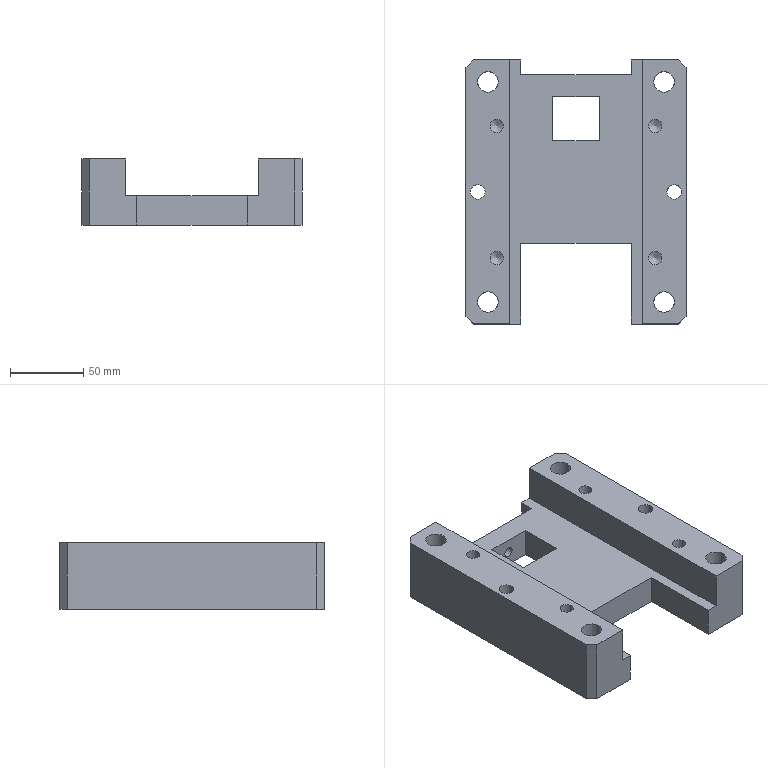Part | NX | features solid 2 | 1 solid | 43 faces | box 150 x 180 x 45 mm | volume 649811 mm3 | plane 27 | cylinder 12 | cone 4 | commonest cylinder face diameters 9 x4 14 x4 10 x2 7 x1 11 x1
STEP:
#1=CARTESIAN_POINT('',(45.,730.,-108.));
#2=VERTEX_POINT('',#1);
#3=CARTESIAN_POINT('',(70.,730.,-108.));
#4=VERTEX_POINT('',#3);
#5=CARTESIAN_POINT('',(45.,730.,-108.));
#6=DIRECTION('',(1.,0.,0.));
#7=VECTOR('',#6,1000.);
#8=LINE('',#5,#7);
#9=EDGE_CURVE('',#2,#4,#8,.T.);
#10=ORIENTED_EDGE('',*,*,#9,.T.);
#11=CARTESIAN_POINT('',(70.,730.,-153.));
#12=VERTEX_POINT('',#11);
#13=CARTESIAN_POINT('',(70.,730.,-153.));
#14=DIRECTION('',(0.,0.,-1.));
#15=VECTOR('',#14,1000.);
#16=LINE('',#13,#15);
#17=EDGE_CURVE('',#4,#12,#16,.T.);
#18=ORIENTED_EDGE('',*,*,#17,.T.);
#19=CARTESIAN_POINT('',(37.5,730.,-153.));
#20=VERTEX_POINT('',#19);
#21=CARTESIAN_POINT('',(75.,730.,-153.));
#22=DIRECTION('',(-1.,0.,0.));
#23=VECTOR('',#22,1000.);
#24=LINE('',#21,#23);
#25=EDGE_CURVE('',#12,#20,#24,.T.);
#26=ORIENTED_EDGE('',*,*,#25,.T.);
#27=CARTESIAN_POINT('',(37.5,730.,-133.));
#28=VERTEX_POINT('',#27);
#29=CARTESIAN_POINT('',(37.5,730.,-153.));
#30=DIRECTION('',(0.,0.,-1.));
#31=VECTOR('',#30,1000.);
#32=LINE('',#29,#31);
#33=EDGE_CURVE('',#28,#20,#32,.T.);
#34=ORIENTED_EDGE('',*,*,#33,.F.);
#35=CARTESIAN_POINT('',(45.,730.,-133.));
#36=VERTEX_POINT('',#35);
#37=CARTESIAN_POINT('',(-45.,730.,-133.));
#38=DIRECTION('',(1.,0.,0.));
#39=VECTOR('',#38,1000.);
#40=LINE('',#37,#39);
#41=EDGE_CURVE('',#28,#36,#40,.T.);
#42=ORIENTED_EDGE('',*,*,#41,.T.);
#43=CARTESIAN_POINT('',(45.,730.,-133.));
#44=DIRECTION('',(0.,0.,1.));
#45=VECTOR('',#44,1000.);
#46=LINE('',#43,#45);
#47=EDGE_CURVE('',#36,#2,#46,.T.);
#48=ORIENTED_EDGE('',*,*,#47,.T.);
#49=EDGE_LOOP('',(#10,#18,#26,#34,#42,#48));
#50=FACE_BOUND('',#49,.T.);
#51=CARTESIAN_POINT('',(45.,730.,-153.));
#52=DIRECTION('',(0.,-1.,0.));
#53=DIRECTION('',(0.,0.,-1.));
#54=AXIS2_PLACEMENT_3D('',#51,#52,#53);
#55=PLANE('',#54);
#56=ADVANCED_FACE('',(#50),#55,.F.);
#57=CARTESIAN_POINT('',(70.,550.,-153.));
#58=VERTEX_POINT('',#57);
#59=CARTESIAN_POINT('',(37.5,550.,-153.));
#60=VERTEX_POINT('',#59);
#61=CARTESIAN_POINT('',(75.,550.,-153.));
#62=DIRECTION('',(-1.,0.,0.));
#63=VECTOR('',#62,1000.);
#64=LINE('',#61,#63);
#65=EDGE_CURVE('',#58,#60,#64,.T.);
#66=ORIENTED_EDGE('',*,*,#65,.F.);
#67=CARTESIAN_POINT('',(70.,550.,-108.));
#68=VERTEX_POINT('',#67);
#69=CARTESIAN_POINT('',(70.,550.,-153.));
#70=DIRECTION('',(0.,0.,1.));
#71=VECTOR('',#70,1000.);
#72=LINE('',#69,#71);
#73=EDGE_CURVE('',#58,#68,#72,.T.);
#74=ORIENTED_EDGE('',*,*,#73,.T.);
#75=CARTESIAN_POINT('',(45.,550.,-108.));
#76=VERTEX_POINT('',#75);
#77=CARTESIAN_POINT('',(45.,550.,-108.));
#78=DIRECTION('',(1.,0.,0.));
#79=VECTOR('',#78,1000.);
#80=LINE('',#77,#79);
#81=EDGE_CURVE('',#76,#68,#80,.T.);
#82=ORIENTED_EDGE('',*,*,#81,.F.);
#83=CARTESIAN_POINT('',(45.,550.,-133.));
#84=VERTEX_POINT('',#83);
#85=CARTESIAN_POINT('',(45.,550.,-133.));
#86=DIRECTION('',(0.,0.,1.));
#87=VECTOR('',#86,1000.);
#88=LINE('',#85,#87);
#89=EDGE_CURVE('',#84,#76,#88,.T.);
#90=ORIENTED_EDGE('',*,*,#89,.F.);
#91=CARTESIAN_POINT('',(37.5,550.,-133.));
#92=VERTEX_POINT('',#91);
#93=CARTESIAN_POINT('',(-45.,550.,-133.));
#94=DIRECTION('',(1.,0.,0.));
#95=VECTOR('',#94,1000.);
#96=LINE('',#93,#95);
#97=EDGE_CURVE('',#92,#84,#96,.T.);
#98=ORIENTED_EDGE('',*,*,#97,.F.);
#99=CARTESIAN_POINT('',(37.5,550.,-153.));
#100=DIRECTION('',(0.,0.,-1.));
#101=VECTOR('',#100,1000.);
#102=LINE('',#99,#101);
#103=EDGE_CURVE('',#92,#60,#102,.T.);
#104=ORIENTED_EDGE('',*,*,#103,.T.);
#105=EDGE_LOOP('',(#66,#74,#82,#90,#98,#104));
#106=FACE_BOUND('',#105,.T.);
#107=CARTESIAN_POINT('',(45.,550.,-153.));
#108=DIRECTION('',(0.,-1.,0.));
#109=DIRECTION('',(0.,0.,-1.));
#110=AXIS2_PLACEMENT_3D('',#107,#108,#109);
#111=PLANE('',#110);
#112=ADVANCED_FACE('',(#106),#111,.T.);
#113=ORIENTED_EDGE('',*,*,#47,.F.);
#114=CARTESIAN_POINT('',(45.,550.,-133.));
#115=DIRECTION('',(0.,1.,0.));
#116=VECTOR('',#115,1000.);
#117=LINE('',#114,#116);
#118=EDGE_CURVE('',#84,#36,#117,.T.);
#119=ORIENTED_EDGE('',*,*,#118,.F.);
#120=ORIENTED_EDGE('',*,*,#89,.T.);
#121=CARTESIAN_POINT('',(45.,550.,-108.));
#122=DIRECTION('',(0.,1.,0.));
#123=VECTOR('',#122,1000.);
#124=LINE('',#121,#123);
#125=EDGE_CURVE('',#76,#2,#124,.T.);
#126=ORIENTED_EDGE('',*,*,#125,.T.);
#127=EDGE_LOOP('',(#113,#119,#120,#126));
#128=FACE_BOUND('',#127,.T.);
#129=CARTESIAN_POINT('',(45.,550.,-133.));
#130=DIRECTION('',(-1.,0.,0.));
#131=DIRECTION('',(0.,0.,-1.));
#132=AXIS2_PLACEMENT_3D('',#129,#130,#131);
#133=PLANE('',#132);
#134=ADVANCED_FACE('',(#128),#133,.T.);
#135=CARTESIAN_POINT('',(58.5,685.,-108.));
#136=VERTEX_POINT('',#135);
#137=CARTESIAN_POINT('',(54.,685.,-108.));
#138=DIRECTION('',(0.,0.,-1.));
#139=DIRECTION('',(1.,0.,0.));
#140=AXIS2_PLACEMENT_3D('',#137,#138,#139);
#141=CIRCLE('',#140,4.5);
#142=EDGE_CURVE('',#136,#136,#141,.T.);
#143=ORIENTED_EDGE('',*,*,#142,.T.);
#144=EDGE_LOOP('',(#143));
#145=FACE_BOUND('',#144,.T.);
#146=CARTESIAN_POINT('',(58.5,595.,-108.));
#147=VERTEX_POINT('',#146);
#148=CARTESIAN_POINT('',(54.,595.,-108.));
#149=DIRECTION('',(0.,0.,-1.));
#150=DIRECTION('',(1.,0.,0.));
#151=AXIS2_PLACEMENT_3D('',#148,#149,#150);
#152=CIRCLE('',#151,4.5);
#153=EDGE_CURVE('',#147,#147,#152,.T.);
#154=ORIENTED_EDGE('',*,*,#153,.T.);
#155=EDGE_LOOP('',(#154));
#156=FACE_BOUND('',#155,.T.);
#157=CARTESIAN_POINT('',(72.,640.,-108.));
#158=VERTEX_POINT('',#157);
#159=CARTESIAN_POINT('',(67.,640.,-108.));
#160=DIRECTION('',(0.,0.,-1.));
#161=DIRECTION('',(1.,0.,0.));
#162=AXIS2_PLACEMENT_3D('',#159,#160,#161);
#163=CIRCLE('',#162,5.);
#164=EDGE_CURVE('',#158,#158,#163,.T.);
#165=ORIENTED_EDGE('',*,*,#164,.T.);
#166=EDGE_LOOP('',(#165));
#167=FACE_BOUND('',#166,.T.);
#168=CARTESIAN_POINT('',(67.,565.,-108.));
#169=VERTEX_POINT('',#168);
#170=CARTESIAN_POINT('',(60.,565.,-108.));
#171=DIRECTION('',(0.,0.,-1.));
#172=DIRECTION('',(1.,0.,0.));
#173=AXIS2_PLACEMENT_3D('',#170,#171,#172);
#174=CIRCLE('',#173,7.);
#175=EDGE_CURVE('',#169,#169,#174,.T.);
#176=ORIENTED_EDGE('',*,*,#175,.T.);
#177=EDGE_LOOP('',(#176));
#178=FACE_BOUND('',#177,.T.);
#179=CARTESIAN_POINT('',(67.,715.,-108.));
#180=VERTEX_POINT('',#179);
#181=CARTESIAN_POINT('',(60.,715.,-108.));
#182=DIRECTION('',(0.,0.,-1.));
#183=DIRECTION('',(1.,0.,0.));
#184=AXIS2_PLACEMENT_3D('',#181,#182,#183);
#185=CIRCLE('',#184,7.);
#186=EDGE_CURVE('',#180,#180,#185,.T.);
#187=ORIENTED_EDGE('',*,*,#186,.T.);
#188=EDGE_LOOP('',(#187));
#189=FACE_BOUND('',#188,.T.);
#190=CARTESIAN_POINT('',(75.,555.,-108.));
#191=VERTEX_POINT('',#190);
#192=CARTESIAN_POINT('',(75.,725.,-108.));
#193=VERTEX_POINT('',#192);
#194=CARTESIAN_POINT('',(75.,550.,-108.));
#195=DIRECTION('',(0.,1.,0.));
#196=VECTOR('',#195,1000.);
#197=LINE('',#194,#196);
#198=EDGE_CURVE('',#191,#193,#197,.T.);
#199=ORIENTED_EDGE('',*,*,#198,.T.);
#200=CARTESIAN_POINT('',(147.5,652.5,-108.));
#201=DIRECTION('',(-0.7071,0.7071,0.));
#202=VECTOR('',#201,1000.);
#203=LINE('',#200,#202);
#204=EDGE_CURVE('',#193,#4,#203,.T.);
#205=ORIENTED_EDGE('',*,*,#204,.T.);
#206=ORIENTED_EDGE('',*,*,#9,.F.);
#207=ORIENTED_EDGE('',*,*,#125,.F.);
#208=ORIENTED_EDGE('',*,*,#81,.T.);
#209=CARTESIAN_POINT('',(57.5,537.5,-108.));
#210=DIRECTION('',(-0.7071,-0.7071,0.));
#211=VECTOR('',#210,1000.);
#212=LINE('',#209,#211);
#213=EDGE_CURVE('',#68,#191,#212,.F.);
#214=ORIENTED_EDGE('',*,*,#213,.T.);
#215=EDGE_LOOP('',(#199,#205,#206,#207,#208,#214));
#216=FACE_BOUND('',#215,.T.);
#217=CARTESIAN_POINT('',(45.,550.,-108.));
#218=DIRECTION('',(0.,0.,1.));
#219=DIRECTION('',(-1.,0.,0.));
#220=AXIS2_PLACEMENT_3D('',#217,#218,#219);
#221=PLANE('',#220);
#222=ADVANCED_FACE('',(#145,#156,#167,#178,#189,#216),#221,.T.);
#223=CARTESIAN_POINT('',(75.,555.,-153.));
#224=VERTEX_POINT('',#223);
#225=CARTESIAN_POINT('',(75.,725.,-153.));
#226=VERTEX_POINT('',#225);
#227=CARTESIAN_POINT('',(75.,550.,-153.));
#228=DIRECTION('',(0.,1.,0.));
#229=VECTOR('',#228,1000.);
#230=LINE('',#227,#229);
#231=EDGE_CURVE('',#224,#226,#230,.T.);
#232=ORIENTED_EDGE('',*,*,#231,.T.);
#233=CARTESIAN_POINT('',(75.,725.,-108.));
#234=DIRECTION('',(0.,0.,1.));
#235=VECTOR('',#234,1000.);
#236=LINE('',#233,#235);
#237=EDGE_CURVE('',#226,#193,#236,.T.);
#238=ORIENTED_EDGE('',*,*,#237,.T.);
#239=ORIENTED_EDGE('',*,*,#198,.F.);
#240=CARTESIAN_POINT('',(75.,555.,-108.));
#241=DIRECTION('',(0.,0.,-1.));
#242=VECTOR('',#241,1000.);
#243=LINE('',#240,#242);
#244=EDGE_CURVE('',#191,#224,#243,.T.);
#245=ORIENTED_EDGE('',*,*,#244,.T.);
#246=EDGE_LOOP('',(#232,#238,#239,#245));
#247=FACE_BOUND('',#246,.T.);
#248=CARTESIAN_POINT('',(75.,550.,-108.));
#249=DIRECTION('',(1.,0.,0.));
#250=DIRECTION('',(0.,0.,1.));
#251=AXIS2_PLACEMENT_3D('',#248,#249,#250);
#252=PLANE('',#251);
#253=ADVANCED_FACE('',(#247),#252,.T.);
#254=CARTESIAN_POINT('',(-67.,645.,-153.));
#255=VERTEX_POINT('',#254);
#256=CARTESIAN_POINT('',(-67.,640.,-153.));
#257=DIRECTION('',(0.,0.,-1.));
#258=DIRECTION('',(0.,1.,0.));
#259=AXIS2_PLACEMENT_3D('',#256,#257,#258);
#260=CIRCLE('',#259,5.);
#261=EDGE_CURVE('',#255,#255,#260,.T.);
#262=ORIENTED_EDGE('',*,*,#261,.F.);
#263=EDGE_LOOP('',(#262));
#264=FACE_BOUND('',#263,.T.);
#265=CARTESIAN_POINT('',(67.,645.,-153.));
#266=VERTEX_POINT('',#265);
#267=CARTESIAN_POINT('',(67.,640.,-153.));
#268=DIRECTION('',(0.,0.,-1.));
#269=DIRECTION('',(0.,1.,0.));
#270=AXIS2_PLACEMENT_3D('',#267,#268,#269);
#271=CIRCLE('',#270,5.);
#272=EDGE_CURVE('',#266,#266,#271,.T.);
#273=ORIENTED_EDGE('',*,*,#272,.F.);
#274=EDGE_LOOP('',(#273));
#275=FACE_BOUND('',#274,.T.);
#276=CARTESIAN_POINT('',(-60.,572.,-153.));
#277=VERTEX_POINT('',#276);
#278=CARTESIAN_POINT('',(-60.,565.,-153.));
#279=DIRECTION('',(0.,0.,-1.));
#280=DIRECTION('',(0.,1.,0.));
#281=AXIS2_PLACEMENT_3D('',#278,#279,#280);
#282=CIRCLE('',#281,7.);
#283=EDGE_CURVE('',#277,#277,#282,.T.);
#284=ORIENTED_EDGE('',*,*,#283,.F.);
#285=EDGE_LOOP('',(#284));
#286=FACE_BOUND('',#285,.T.);
#287=CARTESIAN_POINT('',(-60.,722.,-153.));
#288=VERTEX_POINT('',#287);
#289=CARTESIAN_POINT('',(-60.,715.,-153.));
#290=DIRECTION('',(0.,0.,-1.));
#291=DIRECTION('',(0.,1.,0.));
#292=AXIS2_PLACEMENT_3D('',#289,#290,#291);
#293=CIRCLE('',#292,7.);
#294=EDGE_CURVE('',#288,#288,#293,.T.);
#295=ORIENTED_EDGE('',*,*,#294,.F.);
#296=EDGE_LOOP('',(#295));
#297=FACE_BOUND('',#296,.T.);
#298=CARTESIAN_POINT('',(60.,572.,-153.));
#299=VERTEX_POINT('',#298);
#300=CARTESIAN_POINT('',(60.,565.,-153.));
#301=DIRECTION('',(0.,0.,-1.));
#302=DIRECTION('',(0.,1.,0.));
#303=AXIS2_PLACEMENT_3D('',#300,#301,#302);
#304=CIRCLE('',#303,7.);
#305=EDGE_CURVE('',#299,#299,#304,.T.);
#306=ORIENTED_EDGE('',*,*,#305,.F.);
#307=EDGE_LOOP('',(#306));
#308=FACE_BOUND('',#307,.T.);
#309=CARTESIAN_POINT('',(60.,722.,-153.));
#310=VERTEX_POINT('',#309);
#311=CARTESIAN_POINT('',(60.,715.,-153.));
#312=DIRECTION('',(0.,0.,-1.));
#313=DIRECTION('',(0.,1.,0.));
#314=AXIS2_PLACEMENT_3D('',#311,#312,#313);
#315=CIRCLE('',#314,7.);
#316=EDGE_CURVE('',#310,#310,#315,.T.);
#317=ORIENTED_EDGE('',*,*,#316,.F.);
#318=EDGE_LOOP('',(#317));
#319=FACE_BOUND('',#318,.T.);
#320=CARTESIAN_POINT('',(16.,675.,-153.));
#321=VERTEX_POINT('',#320);
#322=CARTESIAN_POINT('',(16.,705.,-153.));
#323=VERTEX_POINT('',#322);
#324=CARTESIAN_POINT('',(16.,675.,-153.));
#325=DIRECTION('',(0.,1.,0.));
#326=VECTOR('',#325,1000.);
#327=LINE('',#324,#326);
#328=EDGE_CURVE('',#321,#323,#327,.T.);
#329=ORIENTED_EDGE('',*,*,#328,.T.);
#330=CARTESIAN_POINT('',(-16.,705.,-153.));
#331=VERTEX_POINT('',#330);
#332=CARTESIAN_POINT('',(16.,705.,-153.));
#333=DIRECTION('',(-1.,0.,0.));
#334=VECTOR('',#333,1000.);
#335=LINE('',#332,#334);
#336=EDGE_CURVE('',#323,#331,#335,.T.);
#337=ORIENTED_EDGE('',*,*,#336,.T.);
#338=CARTESIAN_POINT('',(-16.,675.,-153.));
#339=VERTEX_POINT('',#338);
#340=CARTESIAN_POINT('',(-16.,675.,-153.));
#341=DIRECTION('',(0.,1.,0.));
#342=VECTOR('',#341,1000.);
#343=LINE('',#340,#342);
#344=EDGE_CURVE('',#339,#331,#343,.T.);
#345=ORIENTED_EDGE('',*,*,#344,.F.);
#346=CARTESIAN_POINT('',(16.,675.,-153.));
#347=DIRECTION('',(-1.,0.,0.));
#348=VECTOR('',#347,1000.);
#349=LINE('',#346,#348);
#350=EDGE_CURVE('',#321,#339,#349,.T.);
#351=ORIENTED_EDGE('',*,*,#350,.F.);
#352=EDGE_LOOP('',(#329,#337,#345,#351));
#353=FACE_BOUND('',#352,.T.);
#354=ORIENTED_EDGE('',*,*,#25,.F.);
#355=CARTESIAN_POINT('',(162.5,637.5,-153.));
#356=DIRECTION('',(0.7071,-0.7071,0.));
#357=VECTOR('',#356,1000.);
#358=LINE('',#355,#357);
#359=EDGE_CURVE('',#12,#226,#358,.T.);
#360=ORIENTED_EDGE('',*,*,#359,.T.);
#361=ORIENTED_EDGE('',*,*,#231,.F.);
#362=CARTESIAN_POINT('',(72.5,552.5,-153.));
#363=DIRECTION('',(0.7071,0.7071,0.));
#364=VECTOR('',#363,1000.);
#365=LINE('',#362,#364);
#366=EDGE_CURVE('',#224,#58,#365,.F.);
#367=ORIENTED_EDGE('',*,*,#366,.T.);
#368=ORIENTED_EDGE('',*,*,#65,.T.);
#369=CARTESIAN_POINT('',(37.5,605.,-153.));
#370=VERTEX_POINT('',#369);
#371=CARTESIAN_POINT('',(37.5,550.,-153.));
#372=DIRECTION('',(0.,1.,0.));
#373=VECTOR('',#372,1000.);
#374=LINE('',#371,#373);
#375=EDGE_CURVE('',#60,#370,#374,.T.);
#376=ORIENTED_EDGE('',*,*,#375,.T.);
#377=CARTESIAN_POINT('',(-37.5,605.,-153.));
#378=VERTEX_POINT('',#377);
#379=CARTESIAN_POINT('',(37.5,605.,-153.));
#380=DIRECTION('',(-1.,0.,0.));
#381=VECTOR('',#380,1000.);
#382=LINE('',#379,#381);
#383=EDGE_CURVE('',#370,#378,#382,.T.);
#384=ORIENTED_EDGE('',*,*,#383,.T.);
#385=CARTESIAN_POINT('',(-37.5,550.,-153.));
#386=VERTEX_POINT('',#385);
#387=CARTESIAN_POINT('',(-37.5,550.,-153.));
#388=DIRECTION('',(0.,1.,0.));
#389=VECTOR('',#388,1000.);
#390=LINE('',#387,#389);
#391=EDGE_CURVE('',#386,#378,#390,.T.);
#392=ORIENTED_EDGE('',*,*,#391,.F.);
#393=CARTESIAN_POINT('',(-70.,550.,-153.));
#394=VERTEX_POINT('',#393);
#395=CARTESIAN_POINT('',(75.,550.,-153.));
#396=DIRECTION('',(-1.,0.,0.));
#397=VECTOR('',#396,1000.);
#398=LINE('',#395,#397);
#399=EDGE_CURVE('',#386,#394,#398,.T.);
#400=ORIENTED_EDGE('',*,*,#399,.T.);
#401=CARTESIAN_POINT('',(-75.,555.,-153.));
#402=VERTEX_POINT('',#401);
#403=CARTESIAN_POINT('',(2.5,477.5,-153.));
#404=DIRECTION('',(0.7071,-0.7071,0.));
#405=VECTOR('',#404,1000.);
#406=LINE('',#403,#405);
#407=EDGE_CURVE('',#394,#402,#406,.F.);
#408=ORIENTED_EDGE('',*,*,#407,.T.);
#409=CARTESIAN_POINT('',(-75.,725.,-153.));
#410=VERTEX_POINT('',#409);
#411=CARTESIAN_POINT('',(-75.,550.,-153.));
#412=DIRECTION('',(0.,1.,0.));
#413=VECTOR('',#412,1000.);
#414=LINE('',#411,#413);
#415=EDGE_CURVE('',#402,#410,#414,.T.);
#416=ORIENTED_EDGE('',*,*,#415,.T.);
#417=CARTESIAN_POINT('',(-70.,730.,-153.));
#418=VERTEX_POINT('',#417);
#419=CARTESIAN_POINT('',(-87.5,712.5,-153.));
#420=DIRECTION('',(0.7071,0.7071,0.));
#421=VECTOR('',#420,1000.);
#422=LINE('',#419,#421);
#423=EDGE_CURVE('',#410,#418,#422,.T.);
#424=ORIENTED_EDGE('',*,*,#423,.T.);
#425=CARTESIAN_POINT('',(-37.5,730.,-153.));
#426=VERTEX_POINT('',#425);
#427=CARTESIAN_POINT('',(75.,730.,-153.));
#428=DIRECTION('',(-1.,0.,0.));
#429=VECTOR('',#428,1000.);
#430=LINE('',#427,#429);
#431=EDGE_CURVE('',#426,#418,#430,.T.);
#432=ORIENTED_EDGE('',*,*,#431,.F.);
#433=CARTESIAN_POINT('',(-37.5,720.,-153.));
#434=VERTEX_POINT('',#433);
#435=CARTESIAN_POINT('',(-37.5,720.,-153.));
#436=DIRECTION('',(0.,1.,0.));
#437=VECTOR('',#436,1000.);
#438=LINE('',#435,#437);
#439=EDGE_CURVE('',#434,#426,#438,.T.);
#440=ORIENTED_EDGE('',*,*,#439,.F.);
#441=CARTESIAN_POINT('',(37.5,720.,-153.));
#442=VERTEX_POINT('',#441);
#443=CARTESIAN_POINT('',(37.5,720.,-153.));
#444=DIRECTION('',(-1.,0.,0.));
#445=VECTOR('',#444,1000.);
#446=LINE('',#443,#445);
#447=EDGE_CURVE('',#442,#434,#446,.T.);
#448=ORIENTED_EDGE('',*,*,#447,.F.);
#449=CARTESIAN_POINT('',(37.5,720.,-153.));
#450=DIRECTION('',(0.,1.,0.));
#451=VECTOR('',#450,1000.);
#452=LINE('',#449,#451);
#453=EDGE_CURVE('',#442,#20,#452,.T.);
#454=ORIENTED_EDGE('',*,*,#453,.T.);
#455=EDGE_LOOP('',(#354,#360,#361,#367,#368,#376,#384,#392,#400,#408,#416,#424,#432,#440,#448,#454));
#456=FACE_BOUND('',#455,.T.);
#457=CARTESIAN_POINT('',(75.,550.,-153.));
#458=DIRECTION('',(0.,0.,-1.));
#459=DIRECTION('',(0.,1.,0.));
#460=AXIS2_PLACEMENT_3D('',#457,#458,#459);
#461=PLANE('',#460);
#462=ADVANCED_FACE('',(#264,#275,#286,#297,#308,#319,#353,#456),#461,.T.);
#463=CARTESIAN_POINT('',(-75.,555.,-108.));
#464=VERTEX_POINT('',#463);
#465=CARTESIAN_POINT('',(-75.,725.,-108.));
#466=VERTEX_POINT('',#465);
#467=CARTESIAN_POINT('',(-75.,550.,-108.));
#468=DIRECTION('',(0.,1.,0.));
#469=VECTOR('',#468,1000.);
#470=LINE('',#467,#469);
#471=EDGE_CURVE('',#464,#466,#470,.T.);
#472=ORIENTED_EDGE('',*,*,#471,.T.);
#473=CARTESIAN_POINT('',(-75.,725.,-153.));
#474=DIRECTION('',(0.,0.,-1.));
#475=VECTOR('',#474,1000.);
#476=LINE('',#473,#475);
#477=EDGE_CURVE('',#466,#410,#476,.T.);
#478=ORIENTED_EDGE('',*,*,#477,.T.);
#479=ORIENTED_EDGE('',*,*,#415,.F.);
#480=CARTESIAN_POINT('',(-75.,555.,-153.));
#481=DIRECTION('',(0.,0.,1.));
#482=VECTOR('',#481,1000.);
#483=LINE('',#480,#482);
#484=EDGE_CURVE('',#402,#464,#483,.T.);
#485=ORIENTED_EDGE('',*,*,#484,.T.);
#486=EDGE_LOOP('',(#472,#478,#479,#485));
#487=FACE_BOUND('',#486,.T.);
#488=CARTESIAN_POINT('',(-75.,550.,-153.));
#489=DIRECTION('',(-1.,0.,0.));
#490=DIRECTION('',(0.,0.,-1.));
#491=AXIS2_PLACEMENT_3D('',#488,#489,#490);
#492=PLANE('',#491);
#493=ADVANCED_FACE('',(#487),#492,.T.);
#494=CARTESIAN_POINT('',(-49.5,685.,-108.));
#495=VERTEX_POINT('',#494);
#496=CARTESIAN_POINT('',(-54.,685.,-108.));
#497=DIRECTION('',(0.,0.,-1.));
#498=DIRECTION('',(1.,0.,0.));
#499=AXIS2_PLACEMENT_3D('',#496,#497,#498);
#500=CIRCLE('',#499,4.5);
#501=EDGE_CURVE('',#495,#495,#500,.T.);
#502=ORIENTED_EDGE('',*,*,#501,.T.);
#503=EDGE_LOOP('',(#502));
#504=FACE_BOUND('',#503,.T.);
#505=CARTESIAN_POINT('',(-49.5,595.,-108.));
#506=VERTEX_POINT('',#505);
#507=CARTESIAN_POINT('',(-54.,595.,-108.));
#508=DIRECTION('',(0.,0.,-1.));
#509=DIRECTION('',(1.,0.,0.));
#510=AXIS2_PLACEMENT_3D('',#507,#508,#509);
#511=CIRCLE('',#510,4.5);
#512=EDGE_CURVE('',#506,#506,#511,.T.);
#513=ORIENTED_EDGE('',*,*,#512,.T.);
#514=EDGE_LOOP('',(#513));
#515=FACE_BOUND('',#514,.T.);
#516=CARTESIAN_POINT('',(-62.,640.,-108.));
#517=VERTEX_POINT('',#516);
#518=CARTESIAN_POINT('',(-67.,640.,-108.));
#519=DIRECTION('',(0.,0.,-1.));
#520=DIRECTION('',(1.,0.,0.));
#521=AXIS2_PLACEMENT_3D('',#518,#519,#520);
#522=CIRCLE('',#521,5.);
#523=EDGE_CURVE('',#517,#517,#522,.T.);
#524=ORIENTED_EDGE('',*,*,#523,.T.);
#525=EDGE_LOOP('',(#524));
#526=FACE_BOUND('',#525,.T.);
#527=CARTESIAN_POINT('',(-53.,565.,-108.));
#528=VERTEX_POINT('',#527);
#529=CARTESIAN_POINT('',(-60.,565.,-108.));
#530=DIRECTION('',(0.,0.,-1.));
#531=DIRECTION('',(1.,0.,0.));
#532=AXIS2_PLACEMENT_3D('',#529,#530,#531);
#533=CIRCLE('',#532,7.);
#534=EDGE_CURVE('',#528,#528,#533,.T.);
#535=ORIENTED_EDGE('',*,*,#534,.T.);
#536=EDGE_LOOP('',(#535));
#537=FACE_BOUND('',#536,.T.);
#538=CARTESIAN_POINT('',(-53.,715.,-108.));
#539=VERTEX_POINT('',#538);
#540=CARTESIAN_POINT('',(-60.,715.,-108.));
#541=DIRECTION('',(0.,0.,-1.));
#542=DIRECTION('',(1.,0.,0.));
#543=AXIS2_PLACEMENT_3D('',#540,#541,#542);
#544=CIRCLE('',#543,7.);
#545=EDGE_CURVE('',#539,#539,#544,.T.);
#546=ORIENTED_EDGE('',*,*,#545,.T.);
#547=EDGE_LOOP('',(#546));
#548=FACE_BOUND('',#547,.T.);
#549=CARTESIAN_POINT('',(-70.,730.,-108.));
#550=VERTEX_POINT('',#549);
#551=CARTESIAN_POINT('',(-45.,730.,-108.));
#552=VERTEX_POINT('',#551);
#553=CARTESIAN_POINT('',(-75.,730.,-108.));
#554=DIRECTION('',(1.,0.,0.));
#555=VECTOR('',#554,1000.);
#556=LINE('',#553,#555);
#557=EDGE_CURVE('',#550,#552,#556,.T.);
#558=ORIENTED_EDGE('',*,*,#557,.F.);
#559=CARTESIAN_POINT('',(-162.5,637.5,-108.));
#560=DIRECTION('',(-0.7071,-0.7071,0.));
#561=VECTOR('',#560,1000.);
#562=LINE('',#559,#561);
#563=EDGE_CURVE('',#550,#466,#562,.T.);
#564=ORIENTED_EDGE('',*,*,#563,.T.);
#565=ORIENTED_EDGE('',*,*,#471,.F.);
#566=CARTESIAN_POINT('',(-70.,550.,-108.));
#567=VERTEX_POINT('',#566);
#568=CARTESIAN_POINT('',(-72.5,552.5,-108.));
#569=DIRECTION('',(-0.7071,0.7071,0.));
#570=VECTOR('',#569,1000.);
#571=LINE('',#568,#570);
#572=EDGE_CURVE('',#464,#567,#571,.F.);
#573=ORIENTED_EDGE('',*,*,#572,.T.);
#574=CARTESIAN_POINT('',(-45.,550.,-108.));
#575=VERTEX_POINT('',#574);
#576=CARTESIAN_POINT('',(-75.,550.,-108.));
#577=DIRECTION('',(1.,0.,0.));
#578=VECTOR('',#577,1000.);
#579=LINE('',#576,#578);
#580=EDGE_CURVE('',#567,#575,#579,.T.);
#581=ORIENTED_EDGE('',*,*,#580,.T.);
#582=CARTESIAN_POINT('',(-45.,550.,-108.));
#583=DIRECTION('',(0.,1.,0.));
#584=VECTOR('',#583,1000.);
#585=LINE('',#582,#584);
#586=EDGE_CURVE('',#575,#552,#585,.T.);
#587=ORIENTED_EDGE('',*,*,#586,.T.);
#588=EDGE_LOOP('',(#558,#564,#565,#573,#581,#587));
#589=FACE_BOUND('',#588,.T.);
#590=CARTESIAN_POINT('',(-75.,550.,-108.));
#591=DIRECTION('',(0.,0.,1.));
#592=DIRECTION('',(0.,-1.,0.));
#593=AXIS2_PLACEMENT_3D('',#590,#591,#592);
#594=PLANE('',#593);
#595=ADVANCED_FACE('',(#504,#515,#526,#537,#548,#589),#594,.T.);
#596=CARTESIAN_POINT('',(-45.,730.,-133.));
#597=VERTEX_POINT('',#596);
#598=CARTESIAN_POINT('',(-45.,730.,-108.));
#599=DIRECTION('',(0.,0.,-1.));
#600=VECTOR('',#599,1000.);
#601=LINE('',#598,#600);
#602=EDGE_CURVE('',#552,#597,#601,.T.);
#603=ORIENTED_EDGE('',*,*,#602,.F.);
#604=ORIENTED_EDGE('',*,*,#586,.F.);
#605=CARTESIAN_POINT('',(-45.,550.,-133.));
#606=VERTEX_POINT('',#605);
#607=CARTESIAN_POINT('',(-45.,550.,-108.));
#608=DIRECTION('',(0.,0.,-1.));
#609=VECTOR('',#608,1000.);
#610=LINE('',#607,#609);
#611=EDGE_CURVE('',#575,#606,#610,.T.);
#612=ORIENTED_EDGE('',*,*,#611,.T.);
#613=CARTESIAN_POINT('',(-45.,550.,-133.));
#614=DIRECTION('',(0.,1.,0.));
#615=VECTOR('',#614,1000.);
#616=LINE('',#613,#615);
#617=EDGE_CURVE('',#606,#597,#616,.T.);
#618=ORIENTED_EDGE('',*,*,#617,.T.);
#619=EDGE_LOOP('',(#603,#604,#612,#618));
#620=FACE_BOUND('',#619,.T.);
#621=CARTESIAN_POINT('',(-45.,550.,-108.));
#622=DIRECTION('',(1.,0.,0.));
#623=DIRECTION('',(0.,0.,1.));
#624=AXIS2_PLACEMENT_3D('',#621,#622,#623);
#625=PLANE('',#624);
#626=ADVANCED_FACE('',(#620),#625,.T.);
#627=CARTESIAN_POINT('',(16.,675.,-133.));
#628=VERTEX_POINT('',#627);
#629=CARTESIAN_POINT('',(16.,705.,-133.));
#630=VERTEX_POINT('',#629);
#631=CARTESIAN_POINT('',(16.,675.,-133.));
#632=DIRECTION('',(0.,1.,0.));
#633=VECTOR('',#632,1000.);
#634=LINE('',#631,#633);
#635=EDGE_CURVE('',#628,#630,#634,.T.);
#636=ORIENTED_EDGE('',*,*,#635,.F.);
#637=CARTESIAN_POINT('',(-16.,675.,-133.));
#638=VERTEX_POINT('',#637);
#639=CARTESIAN_POINT('',(16.,675.,-133.));
#640=DIRECTION('',(-1.,0.,0.));
#641=VECTOR('',#640,1000.);
#642=LINE('',#639,#641);
#643=EDGE_CURVE('',#628,#638,#642,.T.);
#644=ORIENTED_EDGE('',*,*,#643,.T.);
#645=CARTESIAN_POINT('',(-16.,705.,-133.));
#646=VERTEX_POINT('',#645);
#647=CARTESIAN_POINT('',(-16.,675.,-133.));
#648=DIRECTION('',(0.,1.,0.));
#649=VECTOR('',#648,1000.);
#650=LINE('',#647,#649);
#651=EDGE_CURVE('',#638,#646,#650,.T.);
#652=ORIENTED_EDGE('',*,*,#651,.T.);
#653=CARTESIAN_POINT('',(16.,705.,-133.));
#654=DIRECTION('',(-1.,0.,0.));
#655=VECTOR('',#654,1000.);
#656=LINE('',#653,#655);
#657=EDGE_CURVE('',#630,#646,#656,.T.);
#658=ORIENTED_EDGE('',*,*,#657,.F.);
#659=EDGE_LOOP('',(#636,#644,#652,#658));
#660=FACE_BOUND('',#659,.T.);
#661=CARTESIAN_POINT('',(37.5,720.,-133.));
#662=VERTEX_POINT('',#661);
#663=CARTESIAN_POINT('',(37.5,720.,-133.));
#664=DIRECTION('',(0.,1.,0.));
#665=VECTOR('',#664,1000.);
#666=LINE('',#663,#665);
#667=EDGE_CURVE('',#662,#28,#666,.T.);
#668=ORIENTED_EDGE('',*,*,#667,.F.);
#669=CARTESIAN_POINT('',(-37.5,720.,-133.));
#670=VERTEX_POINT('',#669);
#671=CARTESIAN_POINT('',(37.5,720.,-133.));
#672=DIRECTION('',(-1.,0.,0.));
#673=VECTOR('',#672,1000.);
#674=LINE('',#671,#673);
#675=EDGE_CURVE('',#662,#670,#674,.T.);
#676=ORIENTED_EDGE('',*,*,#675,.T.);
#677=CARTESIAN_POINT('',(-37.5,730.,-133.));
#678=VERTEX_POINT('',#677);
#679=CARTESIAN_POINT('',(-37.5,720.,-133.));
#680=DIRECTION('',(0.,1.,0.));
#681=VECTOR('',#680,1000.);
#682=LINE('',#679,#681);
#683=EDGE_CURVE('',#670,#678,#682,.T.);
#684=ORIENTED_EDGE('',*,*,#683,.T.);
#685=CARTESIAN_POINT('',(-45.,730.,-133.));
#686=DIRECTION('',(1.,0.,0.));
#687=VECTOR('',#686,1000.);
#688=LINE('',#685,#687);
#689=EDGE_CURVE('',#597,#678,#688,.T.);
#690=ORIENTED_EDGE('',*,*,#689,.F.);
#691=ORIENTED_EDGE('',*,*,#617,.F.);
#692=CARTESIAN_POINT('',(-37.5,550.,-133.));
#693=VERTEX_POINT('',#692);
#694=CARTESIAN_POINT('',(-45.,550.,-133.));
#695=DIRECTION('',(1.,0.,0.));
#696=VECTOR('',#695,1000.);
#697=LINE('',#694,#696);
#698=EDGE_CURVE('',#606,#693,#697,.T.);
#699=ORIENTED_EDGE('',*,*,#698,.T.);
#700=CARTESIAN_POINT('',(-37.5,605.,-133.));
#701=VERTEX_POINT('',#700);
#702=CARTESIAN_POINT('',(-37.5,550.,-133.));
#703=DIRECTION('',(0.,1.,0.));
#704=VECTOR('',#703,1000.);
#705=LINE('',#702,#704);
#706=EDGE_CURVE('',#693,#701,#705,.T.);
#707=ORIENTED_EDGE('',*,*,#706,.T.);
#708=CARTESIAN_POINT('',(37.5,605.,-133.));
#709=VERTEX_POINT('',#708);
#710=CARTESIAN_POINT('',(37.5,605.,-133.));
#711=DIRECTION('',(-1.,0.,0.));
#712=VECTOR('',#711,1000.);
#713=LINE('',#710,#712);
#714=EDGE_CURVE('',#709,#701,#713,.T.);
#715=ORIENTED_EDGE('',*,*,#714,.F.);
#716=CARTESIAN_POINT('',(37.5,550.,-133.));
#717=DIRECTION('',(0.,1.,0.));
#718=VECTOR('',#717,1000.);
#719=LINE('',#716,#718);
#720=EDGE_CURVE('',#92,#709,#719,.T.);
#721=ORIENTED_EDGE('',*,*,#720,.F.);
#722=ORIENTED_EDGE('',*,*,#97,.T.);
#723=ORIENTED_EDGE('',*,*,#118,.T.);
#724=ORIENTED_EDGE('',*,*,#41,.F.);
#725=EDGE_LOOP('',(#668,#676,#684,#690,#691,#699,#707,#715,#721,#722,#723,#724));
#726=FACE_BOUND('',#725,.T.);
#727=CARTESIAN_POINT('',(-45.,550.,-133.));
#728=DIRECTION('',(0.,0.,1.));
#729=DIRECTION('',(-1.,0.,0.));
#730=AXIS2_PLACEMENT_3D('',#727,#728,#729);
#731=PLANE('',#730);
#732=ADVANCED_FACE('',(#660,#726),#731,.T.);
#733=ORIENTED_EDGE('',*,*,#580,.F.);
#734=CARTESIAN_POINT('',(-70.,550.,-153.));
#735=DIRECTION('',(0.,0.,-1.));
#736=VECTOR('',#735,1000.);
#737=LINE('',#734,#736);
#738=EDGE_CURVE('',#567,#394,#737,.T.);
#739=ORIENTED_EDGE('',*,*,#738,.T.);
#740=ORIENTED_EDGE('',*,*,#399,.F.);
#741=CARTESIAN_POINT('',(-37.5,550.,-153.));
#742=DIRECTION('',(0.,0.,-1.));
#743=VECTOR('',#742,1000.);
#744=LINE('',#741,#743);
#745=EDGE_CURVE('',#693,#386,#744,.T.);
#746=ORIENTED_EDGE('',*,*,#745,.F.);
#747=ORIENTED_EDGE('',*,*,#698,.F.);
#748=ORIENTED_EDGE('',*,*,#611,.F.);
#749=EDGE_LOOP('',(#733,#739,#740,#746,#747,#748));
#750=FACE_BOUND('',#749,.T.);
#751=CARTESIAN_POINT('',(45.,550.,-153.));
#752=DIRECTION('',(0.,-1.,0.));
#753=DIRECTION('',(0.,0.,-1.));
#754=AXIS2_PLACEMENT_3D('',#751,#752,#753);
#755=PLANE('',#754);
#756=ADVANCED_FACE('',(#750),#755,.T.);
#757=ORIENTED_EDGE('',*,*,#431,.T.);
#758=CARTESIAN_POINT('',(-70.,730.,-108.));
#759=DIRECTION('',(0.,0.,1.));
#760=VECTOR('',#759,1000.);
#761=LINE('',#758,#760);
#762=EDGE_CURVE('',#418,#550,#761,.T.);
#763=ORIENTED_EDGE('',*,*,#762,.T.);
#764=ORIENTED_EDGE('',*,*,#557,.T.);
#765=ORIENTED_EDGE('',*,*,#602,.T.);
#766=ORIENTED_EDGE('',*,*,#689,.T.);
#767=CARTESIAN_POINT('',(-37.5,730.,-153.));
#768=DIRECTION('',(0.,0.,-1.));
#769=VECTOR('',#768,1000.);
#770=LINE('',#767,#769);
#771=EDGE_CURVE('',#678,#426,#770,.T.);
#772=ORIENTED_EDGE('',*,*,#771,.T.);
#773=EDGE_LOOP('',(#757,#763,#764,#765,#766,#772));
#774=FACE_BOUND('',#773,.T.);
#775=CARTESIAN_POINT('',(45.,730.,-153.));
#776=DIRECTION('',(0.,-1.,0.));
#777=DIRECTION('',(0.,0.,-1.));
#778=AXIS2_PLACEMENT_3D('',#775,#776,#777);
#779=PLANE('',#778);
#780=ADVANCED_FACE('',(#774),#779,.F.);
#781=ORIENTED_EDGE('',*,*,#720,.T.);
#782=CARTESIAN_POINT('',(37.5,605.,-153.));
#783=DIRECTION('',(0.,0.,-1.));
#784=VECTOR('',#783,1000.);
#785=LINE('',#782,#784);
#786=EDGE_CURVE('',#709,#370,#785,.T.);
#787=ORIENTED_EDGE('',*,*,#786,.T.);
#788=ORIENTED_EDGE('',*,*,#375,.F.);
#789=ORIENTED_EDGE('',*,*,#103,.F.);
#790=EDGE_LOOP('',(#781,#787,#788,#789));
#791=FACE_BOUND('',#790,.T.);
#792=CARTESIAN_POINT('',(37.5,550.,-133.));
#793=DIRECTION('',(1.,0.,0.));
#794=DIRECTION('',(0.,0.,1.));
#795=AXIS2_PLACEMENT_3D('',#792,#793,#794);
#796=PLANE('',#795);
#797=ADVANCED_FACE('',(#791),#796,.F.);
#798=ORIENTED_EDGE('',*,*,#714,.T.);
#799=CARTESIAN_POINT('',(-37.5,605.,-153.));
#800=DIRECTION('',(0.,0.,-1.));
#801=VECTOR('',#800,1000.);
#802=LINE('',#799,#801);
#803=EDGE_CURVE('',#701,#378,#802,.T.);
#804=ORIENTED_EDGE('',*,*,#803,.T.);
#805=ORIENTED_EDGE('',*,*,#383,.F.);
#806=ORIENTED_EDGE('',*,*,#786,.F.);
#807=EDGE_LOOP('',(#798,#804,#805,#806));
#808=FACE_BOUND('',#807,.T.);
#809=CARTESIAN_POINT('',(37.5,605.,-133.));
#810=DIRECTION('',(0.,1.,0.));
#811=DIRECTION('',(0.,0.,-1.));
#812=AXIS2_PLACEMENT_3D('',#809,#810,#811);
#813=PLANE('',#812);
#814=ADVANCED_FACE('',(#808),#813,.F.);
#815=ORIENTED_EDGE('',*,*,#706,.F.);
#816=ORIENTED_EDGE('',*,*,#745,.T.);
#817=ORIENTED_EDGE('',*,*,#391,.T.);
#818=ORIENTED_EDGE('',*,*,#803,.F.);
#819=EDGE_LOOP('',(#815,#816,#817,#818));
#820=FACE_BOUND('',#819,.T.);
#821=CARTESIAN_POINT('',(-37.5,605.,-133.));
#822=DIRECTION('',(-1.,0.,0.));
#823=DIRECTION('',(0.,0.,-1.));
#824=AXIS2_PLACEMENT_3D('',#821,#822,#823);
#825=PLANE('',#824);
#826=ADVANCED_FACE('',(#820),#825,.F.);
#827=ORIENTED_EDGE('',*,*,#667,.T.);
#828=ORIENTED_EDGE('',*,*,#33,.T.);
#829=ORIENTED_EDGE('',*,*,#453,.F.);
#830=CARTESIAN_POINT('',(37.5,720.,-153.));
#831=DIRECTION('',(0.,0.,-1.));
#832=VECTOR('',#831,1000.);
#833=LINE('',#830,#832);
#834=EDGE_CURVE('',#662,#442,#833,.T.);
#835=ORIENTED_EDGE('',*,*,#834,.F.);
#836=EDGE_LOOP('',(#827,#828,#829,#835));
#837=FACE_BOUND('',#836,.T.);
#838=CARTESIAN_POINT('',(37.5,720.,-133.));
#839=DIRECTION('',(1.,0.,0.));
#840=DIRECTION('',(0.,0.,1.));
#841=AXIS2_PLACEMENT_3D('',#838,#839,#840);
#842=PLANE('',#841);
#843=ADVANCED_FACE('',(#837),#842,.F.);
#844=ORIENTED_EDGE('',*,*,#683,.F.);
#845=CARTESIAN_POINT('',(-37.5,720.,-153.));
#846=DIRECTION('',(0.,0.,-1.));
#847=VECTOR('',#846,1000.);
#848=LINE('',#845,#847);
#849=EDGE_CURVE('',#670,#434,#848,.T.);
#850=ORIENTED_EDGE('',*,*,#849,.T.);
#851=ORIENTED_EDGE('',*,*,#439,.T.);
#852=ORIENTED_EDGE('',*,*,#771,.F.);
#853=EDGE_LOOP('',(#844,#850,#851,#852));
#854=FACE_BOUND('',#853,.T.);
#855=CARTESIAN_POINT('',(-37.5,730.,-133.));
#856=DIRECTION('',(-1.,0.,0.));
#857=DIRECTION('',(0.,0.,-1.));
#858=AXIS2_PLACEMENT_3D('',#855,#856,#857);
#859=PLANE('',#858);
#860=ADVANCED_FACE('',(#854),#859,.F.);
#861=CARTESIAN_POINT('',(0.,720.,-148.5));
#862=VERTEX_POINT('',#861);
#863=CARTESIAN_POINT('',(0.,720.,-143.));
#864=DIRECTION('',(0.,-1.,0.));
#865=DIRECTION('',(0.,0.,-1.));
#866=AXIS2_PLACEMENT_3D('',#863,#864,#865);
#867=CIRCLE('',#866,5.5);
#868=EDGE_CURVE('',#862,#862,#867,.T.);
#869=ORIENTED_EDGE('',*,*,#868,.T.);
#870=EDGE_LOOP('',(#869));
#871=FACE_BOUND('',#870,.T.);
#872=ORIENTED_EDGE('',*,*,#834,.T.);
#873=ORIENTED_EDGE('',*,*,#447,.T.);
#874=ORIENTED_EDGE('',*,*,#849,.F.);
#875=ORIENTED_EDGE('',*,*,#675,.F.);
#876=EDGE_LOOP('',(#872,#873,#874,#875));
#877=FACE_BOUND('',#876,.T.);
#878=CARTESIAN_POINT('',(-37.5,720.,-133.));
#879=DIRECTION('',(0.,-1.,0.));
#880=DIRECTION('',(0.,0.,1.));
#881=AXIS2_PLACEMENT_3D('',#878,#879,#880);
#882=PLANE('',#881);
#883=ADVANCED_FACE('',(#871,#877),#882,.F.);
#884=ORIENTED_EDGE('',*,*,#635,.T.);
#885=CARTESIAN_POINT('',(16.,705.,-153.));
#886=DIRECTION('',(0.,0.,-1.));
#887=VECTOR('',#886,1000.);
#888=LINE('',#885,#887);
#889=EDGE_CURVE('',#630,#323,#888,.T.);
#890=ORIENTED_EDGE('',*,*,#889,.T.);
#891=ORIENTED_EDGE('',*,*,#328,.F.);
#892=CARTESIAN_POINT('',(16.,675.,-153.));
#893=DIRECTION('',(0.,0.,-1.));
#894=VECTOR('',#893,1000.);
#895=LINE('',#892,#894);
#896=EDGE_CURVE('',#628,#321,#895,.T.);
#897=ORIENTED_EDGE('',*,*,#896,.F.);
#898=EDGE_LOOP('',(#884,#890,#891,#897));
#899=FACE_BOUND('',#898,.T.);
#900=CARTESIAN_POINT('',(16.,675.,-133.));
#901=DIRECTION('',(1.,0.,0.));
#902=DIRECTION('',(0.,0.,1.));
#903=AXIS2_PLACEMENT_3D('',#900,#901,#902);
#904=PLANE('',#903);
#905=ADVANCED_FACE('',(#899),#904,.F.);
#906=CARTESIAN_POINT('',(0.,705.,-139.5));
#907=VERTEX_POINT('',#906);
#908=CARTESIAN_POINT('',(0.,705.,-143.));
#909=DIRECTION('',(0.,1.,0.));
#910=DIRECTION('',(0.,0.,1.));
#911=AXIS2_PLACEMENT_3D('',#908,#909,#910);
#912=CIRCLE('',#911,3.5);
#913=EDGE_CURVE('',#907,#907,#912,.T.);
#914=ORIENTED_EDGE('',*,*,#913,.T.);
#915=EDGE_LOOP('',(#914));
#916=FACE_BOUND('',#915,.T.);
#917=ORIENTED_EDGE('',*,*,#657,.T.);
#918=CARTESIAN_POINT('',(-16.,705.,-153.));
#919=DIRECTION('',(0.,0.,-1.));
#920=VECTOR('',#919,1000.);
#921=LINE('',#918,#920);
#922=EDGE_CURVE('',#646,#331,#921,.T.);
#923=ORIENTED_EDGE('',*,*,#922,.T.);
#924=ORIENTED_EDGE('',*,*,#336,.F.);
#925=ORIENTED_EDGE('',*,*,#889,.F.);
#926=EDGE_LOOP('',(#917,#923,#924,#925));
#927=FACE_BOUND('',#926,.T.);
#928=CARTESIAN_POINT('',(16.,705.,-133.));
#929=DIRECTION('',(0.,1.,0.));
#930=DIRECTION('',(0.,0.,-1.));
#931=AXIS2_PLACEMENT_3D('',#928,#929,#930);
#932=PLANE('',#931);
#933=ADVANCED_FACE('',(#916,#927),#932,.F.);
#934=ORIENTED_EDGE('',*,*,#651,.F.);
#935=CARTESIAN_POINT('',(-16.,675.,-153.));
#936=DIRECTION('',(0.,0.,-1.));
#937=VECTOR('',#936,1000.);
#938=LINE('',#935,#937);
#939=EDGE_CURVE('',#638,#339,#938,.T.);
#940=ORIENTED_EDGE('',*,*,#939,.T.);
#941=ORIENTED_EDGE('',*,*,#344,.T.);
#942=ORIENTED_EDGE('',*,*,#922,.F.);
#943=EDGE_LOOP('',(#934,#940,#941,#942));
#944=FACE_BOUND('',#943,.T.);
#945=CARTESIAN_POINT('',(-16.,705.,-133.));
#946=DIRECTION('',(-1.,0.,0.));
#947=DIRECTION('',(0.,0.,-1.));
#948=AXIS2_PLACEMENT_3D('',#945,#946,#947);
#949=PLANE('',#948);
#950=ADVANCED_FACE('',(#944),#949,.F.);
#951=ORIENTED_EDGE('',*,*,#896,.T.);
#952=ORIENTED_EDGE('',*,*,#350,.T.);
#953=ORIENTED_EDGE('',*,*,#939,.F.);
#954=ORIENTED_EDGE('',*,*,#643,.F.);
#955=EDGE_LOOP('',(#951,#952,#953,#954));
#956=FACE_BOUND('',#955,.T.);
#957=CARTESIAN_POINT('',(-16.,675.,-133.));
#958=DIRECTION('',(0.,-1.,0.));
#959=DIRECTION('',(0.,0.,1.));
#960=AXIS2_PLACEMENT_3D('',#957,#958,#959);
#961=PLANE('',#960);
#962=ADVANCED_FACE('',(#956),#961,.F.);
#963=ORIENTED_EDGE('',*,*,#316,.T.);
#964=EDGE_LOOP('',(#963));
#965=FACE_BOUND('',#964,.T.);
#966=ORIENTED_EDGE('',*,*,#186,.F.);
#967=EDGE_LOOP('',(#966));
#968=FACE_BOUND('',#967,.T.);
#969=CARTESIAN_POINT('',(60.,715.,-108.));
#970=DIRECTION('',(0.,0.,-1.));
#971=DIRECTION('',(1.,0.,0.));
#972=AXIS2_PLACEMENT_3D('',#969,#970,#971);
#973=CYLINDRICAL_SURFACE('',#972,7.);
#974=ADVANCED_FACE('',(#965,#968),#973,.F.);
#975=ORIENTED_EDGE('',*,*,#305,.T.);
#976=EDGE_LOOP('',(#975));
#977=FACE_BOUND('',#976,.T.);
#978=ORIENTED_EDGE('',*,*,#175,.F.);
#979=EDGE_LOOP('',(#978));
#980=FACE_BOUND('',#979,.T.);
#981=CARTESIAN_POINT('',(60.,565.,-108.));
#982=DIRECTION('',(0.,0.,-1.));
#983=DIRECTION('',(1.,0.,0.));
#984=AXIS2_PLACEMENT_3D('',#981,#982,#983);
#985=CYLINDRICAL_SURFACE('',#984,7.);
#986=ADVANCED_FACE('',(#977,#980),#985,.F.);
#987=ORIENTED_EDGE('',*,*,#294,.T.);
#988=EDGE_LOOP('',(#987));
#989=FACE_BOUND('',#988,.T.);
#990=ORIENTED_EDGE('',*,*,#545,.F.);
#991=EDGE_LOOP('',(#990));
#992=FACE_BOUND('',#991,.T.);
#993=CARTESIAN_POINT('',(-60.,715.,-108.));
#994=DIRECTION('',(0.,0.,-1.));
#995=DIRECTION('',(1.,0.,0.));
#996=AXIS2_PLACEMENT_3D('',#993,#994,#995);
#997=CYLINDRICAL_SURFACE('',#996,7.);
#998=ADVANCED_FACE('',(#989,#992),#997,.F.);
#999=ORIENTED_EDGE('',*,*,#283,.T.);
#1000=EDGE_LOOP('',(#999));
#1001=FACE_BOUND('',#1000,.T.);
#1002=ORIENTED_EDGE('',*,*,#534,.F.);
#1003=EDGE_LOOP('',(#1002));
#1004=FACE_BOUND('',#1003,.T.);
#1005=CARTESIAN_POINT('',(-60.,565.,-108.));
#1006=DIRECTION('',(0.,0.,-1.));
#1007=DIRECTION('',(1.,0.,0.));
#1008=AXIS2_PLACEMENT_3D('',#1005,#1006,#1007);
#1009=CYLINDRICAL_SURFACE('',#1008,7.);
#1010=ADVANCED_FACE('',(#1001,#1004),#1009,.F.);
#1011=ORIENTED_EDGE('',*,*,#272,.T.);
#1012=EDGE_LOOP('',(#1011));
#1013=FACE_BOUND('',#1012,.T.);
#1014=ORIENTED_EDGE('',*,*,#164,.F.);
#1015=EDGE_LOOP('',(#1014));
#1016=FACE_BOUND('',#1015,.T.);
#1017=CARTESIAN_POINT('',(67.,640.,-108.));
#1018=DIRECTION('',(0.,0.,-1.));
#1019=DIRECTION('',(1.,0.,0.));
#1020=AXIS2_PLACEMENT_3D('',#1017,#1018,#1019);
#1021=CYLINDRICAL_SURFACE('',#1020,5.);
#1022=ADVANCED_FACE('',(#1013,#1016),#1021,.F.);
#1023=ORIENTED_EDGE('',*,*,#261,.T.);
#1024=EDGE_LOOP('',(#1023));
#1025=FACE_BOUND('',#1024,.T.);
#1026=ORIENTED_EDGE('',*,*,#523,.F.);
#1027=EDGE_LOOP('',(#1026));
#1028=FACE_BOUND('',#1027,.T.);
#1029=CARTESIAN_POINT('',(-67.,640.,-108.));
#1030=DIRECTION('',(0.,0.,-1.));
#1031=DIRECTION('',(1.,0.,0.));
#1032=AXIS2_PLACEMENT_3D('',#1029,#1030,#1031);
#1033=CYLINDRICAL_SURFACE('',#1032,5.);
#1034=ADVANCED_FACE('',(#1025,#1028),#1033,.F.);
#1035=ORIENTED_EDGE('',*,*,#204,.F.);
#1036=ORIENTED_EDGE('',*,*,#237,.F.);
#1037=ORIENTED_EDGE('',*,*,#359,.F.);
#1038=ORIENTED_EDGE('',*,*,#17,.F.);
#1039=EDGE_LOOP('',(#1035,#1036,#1037,#1038));
#1040=FACE_BOUND('',#1039,.T.);
#1041=CARTESIAN_POINT('',(70.,730.,-153.));
#1042=DIRECTION('',(0.7071,0.7071,0.));
#1043=DIRECTION('',(-0.7071,0.7071,0.));
#1044=AXIS2_PLACEMENT_3D('',#1041,#1042,#1043);
#1045=PLANE('',#1044);
#1046=ADVANCED_FACE('',(#1040),#1045,.T.);
#1047=ORIENTED_EDGE('',*,*,#213,.F.);
#1048=ORIENTED_EDGE('',*,*,#73,.F.);
#1049=ORIENTED_EDGE('',*,*,#366,.F.);
#1050=ORIENTED_EDGE('',*,*,#244,.F.);
#1051=EDGE_LOOP('',(#1047,#1048,#1049,#1050));
#1052=FACE_BOUND('',#1051,.T.);
#1053=CARTESIAN_POINT('',(75.,555.,-108.));
#1054=DIRECTION('',(-0.7071,0.7071,0.));
#1055=DIRECTION('',(-0.7071,-0.7071,0.));
#1056=AXIS2_PLACEMENT_3D('',#1053,#1054,#1055);
#1057=PLANE('',#1056);
#1058=ADVANCED_FACE('',(#1052),#1057,.F.);
#1059=ORIENTED_EDGE('',*,*,#423,.F.);
#1060=ORIENTED_EDGE('',*,*,#477,.F.);
#1061=ORIENTED_EDGE('',*,*,#563,.F.);
#1062=ORIENTED_EDGE('',*,*,#762,.F.);
#1063=EDGE_LOOP('',(#1059,#1060,#1061,#1062));
#1064=FACE_BOUND('',#1063,.T.);
#1065=CARTESIAN_POINT('',(-70.,730.,-153.));
#1066=DIRECTION('',(-0.7071,0.7071,0.));
#1067=DIRECTION('',(-0.7071,-0.7071,0.));
#1068=AXIS2_PLACEMENT_3D('',#1065,#1066,#1067);
#1069=PLANE('',#1068);
#1070=ADVANCED_FACE('',(#1064),#1069,.T.);
#1071=ORIENTED_EDGE('',*,*,#407,.F.);
#1072=ORIENTED_EDGE('',*,*,#738,.F.);
#1073=ORIENTED_EDGE('',*,*,#572,.F.);
#1074=ORIENTED_EDGE('',*,*,#484,.F.);
#1075=EDGE_LOOP('',(#1071,#1072,#1073,#1074));
#1076=FACE_BOUND('',#1075,.T.);
#1077=CARTESIAN_POINT('',(-75.,555.,-153.));
#1078=DIRECTION('',(0.7071,0.7071,0.));
#1079=DIRECTION('',(-0.7071,0.7071,0.));
#1080=AXIS2_PLACEMENT_3D('',#1077,#1078,#1079);
#1081=PLANE('',#1080);
#1082=ADVANCED_FACE('',(#1076),#1081,.F.);
#1083=CARTESIAN_POINT('',(0.,710.,-146.5));
#1084=VERTEX_POINT('',#1083);
#1085=CARTESIAN_POINT('',(0.,710.,-143.));
#1086=DIRECTION('',(0.,-1.,0.));
#1087=DIRECTION('',(0.,0.,-1.));
#1088=AXIS2_PLACEMENT_3D('',#1085,#1086,#1087);
#1089=CIRCLE('',#1088,3.5);
#1090=EDGE_CURVE('',#1084,#1084,#1089,.T.);
#1091=ORIENTED_EDGE('',*,*,#1090,.F.);
#1092=EDGE_LOOP('',(#1091));
#1093=FACE_BOUND('',#1092,.T.);
#1094=ORIENTED_EDGE('',*,*,#913,.F.);
#1095=EDGE_LOOP('',(#1094));
#1096=FACE_BOUND('',#1095,.T.);
#1097=CARTESIAN_POINT('',(0.,-494270.,-143.));
#1098=DIRECTION('',(0.,-1.,0.));
#1099=DIRECTION('',(0.,0.,-1.));
#1100=AXIS2_PLACEMENT_3D('',#1097,#1098,#1099);
#1101=CYLINDRICAL_SURFACE('',#1100,3.5);
#1102=ADVANCED_FACE('',(#1093,#1096),#1101,.F.);
#1103=ORIENTED_EDGE('',*,*,#1090,.T.);
#1104=EDGE_LOOP('',(#1103));
#1105=FACE_BOUND('',#1104,.T.);
#1106=CARTESIAN_POINT('',(0.,710.,-148.5));
#1107=VERTEX_POINT('',#1106);
#1108=CARTESIAN_POINT('',(0.,710.,-143.));
#1109=DIRECTION('',(0.,-1.,0.));
#1110=DIRECTION('',(0.,0.,-1.));
#1111=AXIS2_PLACEMENT_3D('',#1108,#1109,#1110);
#1112=CIRCLE('',#1111,5.5);
#1113=EDGE_CURVE('',#1107,#1107,#1112,.T.);
#1114=ORIENTED_EDGE('',*,*,#1113,.F.);
#1115=EDGE_LOOP('',(#1114));
#1116=FACE_BOUND('',#1115,.T.);
#1117=CARTESIAN_POINT('',(0.,710.,-143.));
#1118=DIRECTION('',(0.,-1.,0.));
#1119=DIRECTION('',(0.,0.,-1.));
#1120=AXIS2_PLACEMENT_3D('',#1117,#1118,#1119);
#1121=PLANE('',#1120);
#1122=ADVANCED_FACE('',(#1105,#1116),#1121,.F.);
#1123=ORIENTED_EDGE('',*,*,#1113,.T.);
#1124=EDGE_LOOP('',(#1123));
#1125=FACE_BOUND('',#1124,.T.);
#1126=ORIENTED_EDGE('',*,*,#868,.F.);
#1127=EDGE_LOOP('',(#1126));
#1128=FACE_BOUND('',#1127,.T.);
#1129=CARTESIAN_POINT('',(0.,720.,-143.));
#1130=DIRECTION('',(0.,-1.,0.));
#1131=DIRECTION('',(0.,0.,-1.));
#1132=AXIS2_PLACEMENT_3D('',#1129,#1130,#1131);
#1133=CYLINDRICAL_SURFACE('',#1132,5.5);
#1134=ADVANCED_FACE('',(#1125,#1128),#1133,.F.);
#1135=CARTESIAN_POINT('',(58.5,595.,-128.));
#1136=VERTEX_POINT('',#1135);
#1137=CARTESIAN_POINT('',(54.,595.,-128.));
#1138=DIRECTION('',(0.,0.,-1.));
#1139=DIRECTION('',(1.,0.,0.));
#1140=AXIS2_PLACEMENT_3D('',#1137,#1138,#1139);
#1141=CIRCLE('',#1140,4.5);
#1142=EDGE_CURVE('',#1136,#1136,#1141,.T.);
#1143=ORIENTED_EDGE('',*,*,#1142,.F.);
#1144=EDGE_LOOP('',(#1143));
#1145=FACE_BOUND('',#1144,.T.);
#1146=CARTESIAN_POINT('',(54.,595.,-130.704));
#1147=VERTEX_POINT('',#1146);
#1148=VERTEX_LOOP('',#1147);
#1149=FACE_BOUND('',#1148,.T.);
#1150=CARTESIAN_POINT('',(54.,595.,-128.));
#1151=DIRECTION('',(0.,0.,1.));
#1152=DIRECTION('',(-1.,0.,0.));
#1153=AXIS2_PLACEMENT_3D('',#1150,#1151,#1152);
#1154=CONICAL_SURFACE('',#1153,4.5,1.03);
#1155=ADVANCED_FACE('',(#1145,#1149),#1154,.F.);
#1156=ORIENTED_EDGE('',*,*,#1142,.T.);
#1157=EDGE_LOOP('',(#1156));
#1158=FACE_BOUND('',#1157,.T.);
#1159=ORIENTED_EDGE('',*,*,#153,.F.);
#1160=EDGE_LOOP('',(#1159));
#1161=FACE_BOUND('',#1160,.T.);
#1162=CARTESIAN_POINT('',(54.,595.,-108.));
#1163=DIRECTION('',(0.,0.,-1.));
#1164=DIRECTION('',(1.,0.,0.));
#1165=AXIS2_PLACEMENT_3D('',#1162,#1163,#1164);
#1166=CYLINDRICAL_SURFACE('',#1165,4.5);
#1167=ADVANCED_FACE('',(#1158,#1161),#1166,.F.);
#1168=CARTESIAN_POINT('',(-49.5,595.,-128.));
#1169=VERTEX_POINT('',#1168);
#1170=CARTESIAN_POINT('',(-54.,595.,-128.));
#1171=DIRECTION('',(0.,0.,-1.));
#1172=DIRECTION('',(1.,0.,0.));
#1173=AXIS2_PLACEMENT_3D('',#1170,#1171,#1172);
#1174=CIRCLE('',#1173,4.5);
#1175=EDGE_CURVE('',#1169,#1169,#1174,.T.);
#1176=ORIENTED_EDGE('',*,*,#1175,.F.);
#1177=EDGE_LOOP('',(#1176));
#1178=FACE_BOUND('',#1177,.T.);
#1179=CARTESIAN_POINT('',(-54.,595.,-130.704));
#1180=VERTEX_POINT('',#1179);
#1181=VERTEX_LOOP('',#1180);
#1182=FACE_BOUND('',#1181,.T.);
#1183=CARTESIAN_POINT('',(-54.,595.,-128.));
#1184=DIRECTION('',(0.,0.,1.));
#1185=DIRECTION('',(-1.,0.,0.));
#1186=AXIS2_PLACEMENT_3D('',#1183,#1184,#1185);
#1187=CONICAL_SURFACE('',#1186,4.5,1.03);
#1188=ADVANCED_FACE('',(#1178,#1182),#1187,.F.);
#1189=ORIENTED_EDGE('',*,*,#1175,.T.);
#1190=EDGE_LOOP('',(#1189));
#1191=FACE_BOUND('',#1190,.T.);
#1192=ORIENTED_EDGE('',*,*,#512,.F.);
#1193=EDGE_LOOP('',(#1192));
#1194=FACE_BOUND('',#1193,.T.);
#1195=CARTESIAN_POINT('',(-54.,595.,-108.));
#1196=DIRECTION('',(0.,0.,-1.));
#1197=DIRECTION('',(1.,0.,0.));
#1198=AXIS2_PLACEMENT_3D('',#1195,#1196,#1197);
#1199=CYLINDRICAL_SURFACE('',#1198,4.5);
#1200=ADVANCED_FACE('',(#1191,#1194),#1199,.F.);
#1201=CARTESIAN_POINT('',(58.5,685.,-128.));
#1202=VERTEX_POINT('',#1201);
#1203=CARTESIAN_POINT('',(54.,685.,-128.));
#1204=DIRECTION('',(0.,0.,-1.));
#1205=DIRECTION('',(1.,0.,0.));
#1206=AXIS2_PLACEMENT_3D('',#1203,#1204,#1205);
#1207=CIRCLE('',#1206,4.5);
#1208=EDGE_CURVE('',#1202,#1202,#1207,.T.);
#1209=ORIENTED_EDGE('',*,*,#1208,.F.);
#1210=EDGE_LOOP('',(#1209));
#1211=FACE_BOUND('',#1210,.T.);
#1212=CARTESIAN_POINT('',(54.,685.,-130.704));
#1213=VERTEX_POINT('',#1212);
#1214=VERTEX_LOOP('',#1213);
#1215=FACE_BOUND('',#1214,.T.);
#1216=CARTESIAN_POINT('',(54.,685.,-128.));
#1217=DIRECTION('',(0.,0.,1.));
#1218=DIRECTION('',(-1.,0.,0.));
#1219=AXIS2_PLACEMENT_3D('',#1216,#1217,#1218);
#1220=CONICAL_SURFACE('',#1219,4.5,1.03);
#1221=ADVANCED_FACE('',(#1211,#1215),#1220,.F.);
#1222=ORIENTED_EDGE('',*,*,#1208,.T.);
#1223=EDGE_LOOP('',(#1222));
#1224=FACE_BOUND('',#1223,.T.);
#1225=ORIENTED_EDGE('',*,*,#142,.F.);
#1226=EDGE_LOOP('',(#1225));
#1227=FACE_BOUND('',#1226,.T.);
#1228=CARTESIAN_POINT('',(54.,685.,-108.));
#1229=DIRECTION('',(0.,0.,-1.));
#1230=DIRECTION('',(1.,0.,0.));
#1231=AXIS2_PLACEMENT_3D('',#1228,#1229,#1230);
#1232=CYLINDRICAL_SURFACE('',#1231,4.5);
#1233=ADVANCED_FACE('',(#1224,#1227),#1232,.F.);
#1234=CARTESIAN_POINT('',(-49.5,685.,-128.));
#1235=VERTEX_POINT('',#1234);
#1236=CARTESIAN_POINT('',(-54.,685.,-128.));
#1237=DIRECTION('',(0.,0.,-1.));
#1238=DIRECTION('',(1.,0.,0.));
#1239=AXIS2_PLACEMENT_3D('',#1236,#1237,#1238);
#1240=CIRCLE('',#1239,4.5);
#1241=EDGE_CURVE('',#1235,#1235,#1240,.T.);
#1242=ORIENTED_EDGE('',*,*,#1241,.F.);
#1243=EDGE_LOOP('',(#1242));
#1244=FACE_BOUND('',#1243,.T.);
#1245=CARTESIAN_POINT('',(-54.,685.,-130.704));
#1246=VERTEX_POINT('',#1245);
#1247=VERTEX_LOOP('',#1246);
#1248=FACE_BOUND('',#1247,.T.);
#1249=CARTESIAN_POINT('',(-54.,685.,-128.));
#1250=DIRECTION('',(0.,0.,1.));
#1251=DIRECTION('',(-1.,0.,0.));
#1252=AXIS2_PLACEMENT_3D('',#1249,#1250,#1251);
#1253=CONICAL_SURFACE('',#1252,4.5,1.03);
#1254=ADVANCED_FACE('',(#1244,#1248),#1253,.F.);
#1255=ORIENTED_EDGE('',*,*,#1241,.T.);
#1256=EDGE_LOOP('',(#1255));
#1257=FACE_BOUND('',#1256,.T.);
#1258=ORIENTED_EDGE('',*,*,#501,.F.);
#1259=EDGE_LOOP('',(#1258));
#1260=FACE_BOUND('',#1259,.T.);
#1261=CARTESIAN_POINT('',(-54.,685.,-108.));
#1262=DIRECTION('',(0.,0.,-1.));
#1263=DIRECTION('',(1.,0.,0.));
#1264=AXIS2_PLACEMENT_3D('',#1261,#1262,#1263);
#1265=CYLINDRICAL_SURFACE('',#1264,4.5);
#1266=ADVANCED_FACE('',(#1257,#1260),#1265,.F.);
#1267=CLOSED_SHELL('',(#56,#112,#134,#222,#253,#462,#493,#595,#626,#732,#756,#780,#797,#814,#826,#843,#860,#883,#905,#933,#950,#962,#974,#986,#998,#1010,#1022,#1034,#1046,#1058,#1070,#1082,#1102,#1122,#1134,#1155,#1167,#1188,#1200,#1221,#1233,#1254,#1266));
#1268=MANIFOLD_SOLID_BREP('',#1267);
#1269=(LENGTH_UNIT()NAMED_UNIT(*)SI_UNIT(.MILLI.,.METRE.));
#1270=UNCERTAINTY_MEASURE_WITH_UNIT(LENGTH_MEASURE(0.00001),#1269,'','');
#1271=(NAMED_UNIT(*)PLANE_ANGLE_UNIT()SI_UNIT($,.RADIAN.));
#1272=(NAMED_UNIT(*)SI_UNIT($,.STERADIAN.)SOLID_ANGLE_UNIT());
#1273=(GEOMETRIC_REPRESENTATION_CONTEXT(3)GLOBAL_UNCERTAINTY_ASSIGNED_CONTEXT((#1270))GLOBAL_UNIT_ASSIGNED_CONTEXT((#1269,#1271,#1272))REPRESENTATION_CONTEXT('',''));
#1274=ADVANCED_BREP_SHAPE_REPRESENTATION('',(#1268),#1273);